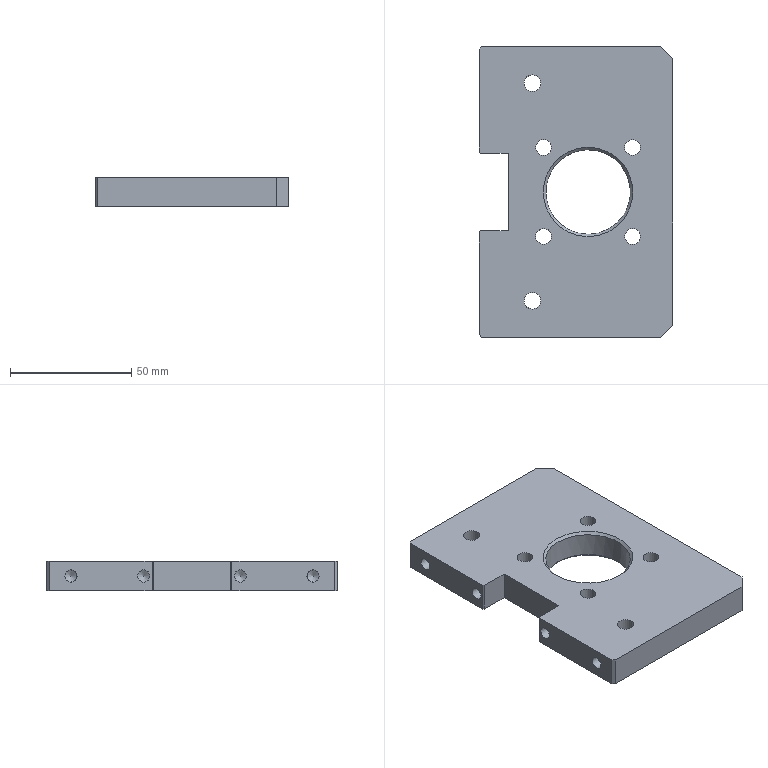NC program | NX | posted with a generic post | part box 80 x 120 x 12 mm
Whole program:
N10 G17 G21 G94 G90
(DRILLING_COPY , TOOL : D8A45)
N12 T06 M6
N14 G54
N16 G17 G0 G90 X-45. Y-18. B0. C0. S3500 M3
N18 G43 Z30. H6
N20 G94 G81 G98 Z-2.6 F250. R3.
N22 X0. Y5.
N24 X18.385 Y23.385
N26 Y-13.385
N28 X-18.385
N30 Y23.385
N32 X45. Y-18.
N34 G80
N36 G0 X45. Y-18. Z30.
N38 M5
(DRILLING_1_COPY , TOOL : 6.8ZT)
N40 T15 M6
N42 G54
N44 G17 G0 G90 X-45. Y-18. B0. C0. S2000 M3
N46 G43 Z30. H15
N48 G94 G83 G98 Z-15.543 F200. Q3. R3.
N50 X45.
N52 G80
N54 G0 X45. Y-18. Z30.
N56 M5
(DRILLING_1_COPY_COPY , TOOL : 6.5ZT)
N58 T22 M6
N60 G54
N62 G17 G0 G90 X18.385 Y23.385 B0. C0. S2000 M3
N64 G43 Z30. H22
N66 G94 G83 G98 Z-15.453 F200. Q3. R3.
N68 Y-13.385
N70 X-18.385
N72 Y23.385
N74 G80
N76 G0 X-18.385 Y23.385 Z30.
N78 M5
(HOLE_MILLING , TOOL : D10)
N80 T04 M6
N82 G54
N84 G17 G0 G90 X0. Y5. B0. C0. S7000 M3
N86 G43 Z30. H4
N88 Z0.5
N90 G94 G3 X3.1 Y8.1 R3.1 F2000.
N92 X0. Y11.2 R3.1
N94 X0. Y11.2 Z-0.5 I0. J-6.2
N96 X0. Y11.2 Z-1.5 I0. J-6.2
N98 X0. Y11.2 Z-2.5 I0. J-6.2
N100 X0. Y11.2 Z-3.5 I0. J-6.2
N102 X0. Y11.2 Z-4.5 I0. J-6.2
N104 X0. Y11.2 Z-5.5 I0. J-6.2
N106 X0. Y11.2 Z-6.5 I0. J-6.2
N108 X0. Y11.2 Z-7.5 I0. J-6.2
N110 X0. Y11.2 Z-8.5 I0. J-6.2
N112 X0. Y11.2 Z-9.5 I0. J-6.2
N114 X0. Y11.2 Z-10.5 I0. J-6.2
N116 X0. Y11.2 Z-11.5 I0. J-6.2
N118 X0. Y-1.2 Z-12. I0. J-6.2
N120 X6.2 Y5. R6.2
N122 X0. Y-1.2 R-6.2
N124 X3.1 Y1.9 R3.1
N126 X0. Y5. R3.1
N128 G0 Z0.5
N130 G3 X6.2 Y11.2 R6.2
N132 X0. Y17.4 R6.2
N134 X0. Y17.4 Z-0.5 I0. J-12.4
N136 X0. Y17.4 Z-1.5 I0. J-12.4
N138 X0. Y17.4 Z-2.5 I0. J-12.4
N140 X0. Y17.4 Z-3.5 I0. J-12.4
N142 X0. Y17.4 Z-4.5 I0. J-12.4
N144 X0. Y17.4 Z-5.5 I0. J-12.4
N146 X0. Y17.4 Z-6.5 I0. J-12.4
N148 X0. Y17.4 Z-7.5 I0. J-12.4
N150 X0. Y17.4 Z-8.5 I0. J-12.4
N152 X0. Y17.4 Z-9.5 I0. J-12.4
N154 X0. Y17.4 Z-10.5 I0. J-12.4
N156 X0. Y17.4 Z-11.5 I0. J-12.4
N158 X0. Y-7.4 Z-12. I0. J-12.4
N160 X12.4 Y5. R12.4
N162 X0. Y-7.4 R-12.4
N164 X6.2 Y-1.2 R6.2
N166 X0. Y5. R6.2
N168 G0 Z30.
(HOLE_MILLING_COPY , TOOL : D10)
N170 Z0.5
N172 G1 X2.609 Y14.031 F1200.
N174 G3 X0. Y17.5 R2.716
N176 X0. Y17.5 Z-3. I0. J-12.5
N178 X0. Y17.5 Z-6.5 I0. J-12.5
N180 X0. Y17.5 Z-10. I0. J-12.5
N182 X5.424 Y-6.262 Z-12. R-12.5
N184 X11.262 Y10.424 R12.5
N186 X5.424 Y-6.262 R-12.5
N188 X6.269 Y-2.004 R2.716
N190 G1 X0. Y5.
N192 G0 Z30.
N194 M5
(PLANAR_MILL_COPY , TOOL : D8A45)
N196 T06 M6
N198 G54
N200 G17 G0 G90 X-46.5 Y-17.134 B0. C0. S7000 M3
N202 G43 Z30. H6
N204 Z0.
N206 G94 G1 Z-1.5 F1250.
N208 G3 X-47. Y-18. R1.
N210 X-45. Y-20. R2.
N212 X-47. Y-18. R-2.
N214 X-46.5 Y-18.866 R1.
N216 G1 Z0.
N218 G0 Z30.
N220 X-19.251 Y-14.735
N222 Z0.
N224 G1 Z-1.5
N226 G3 X-18.385 Y-15.235 R1.
N228 X-16.535 Y-13.385 R1.85
N230 X-18.385 Y-15.235 R-1.85
N232 X-17.519 Y-14.735 R1.
N234 G1 Z0.
N236 G0 Z30.
N238 X-0.866 Y41.9
N240 Z0.
N242 G1 Z-1.5
N244 G3 X0. Y41.4 R1.
N246 G1 X55.
N248 G2 X55.99 Y40.99 R1.4
N250 G1 X60.99 Y35.99
N252 G2 X61.4 Y35. R1.4
N254 G1 Y-39.
N256 G2 X60.99 Y-39.99 R1.4
N258 G1 X59.99 Y-40.99
N260 G2 X59. Y-41.4 R1.4
N262 G1 X16.5
N264 G2 X15.51 Y-40.99 R1.4
N266 G1 X15.01 Y-40.49
N268 G2 X14.6 Y-39.5 R1.4
N270 G1 Y-29.4
N272 X-14.6
N274 Y-39.5
N276 G2 X-15.01 Y-40.49 R1.4
N278 G1 X-15.51 Y-40.99
N280 G2 X-16.5 Y-41.4 R1.4
N282 G1 X-59.
N284 G2 X-59.99 Y-40.99 R1.4
N286 G1 X-60.99 Y-39.99
N288 G2 X-61.4 Y-39. R1.4
N290 G1 Y35.
N292 G2 X-60.99 Y35.99 R1.4
N294 G1 X-55.99 Y40.99
N296 G2 X-55. Y41.4 R1.4
N298 G1 X0.
N300 G3 X0.866 Y41.9 R1.
N302 G1 Z0.
N304 G0 Z30.
N306 Y21.6
N308 Z0.
N310 G1 Z-1.5
N312 G3 X0. Y22.1 R1.
N314 X-17.1 Y5. R17.1
N316 X0. Y22.1 R-17.1
N318 X-0.866 Y21.6 R1.
N320 G1 Z0.
N322 G0 Z30.
N324 X-17.519 Y24.735
N326 Z0.
N328 G1 Z-1.5
N330 G3 X-18.385 Y25.235 R1.
N332 X-20.235 Y23.385 R1.85
N334 X-18.385 Y25.235 R-1.85
N336 X-19.251 Y24.735 R1.
N338 G1 Z0.
N340 G0 Z30.
N342 X19.251
N344 Z0.
N346 G1 Z-1.5
N348 G3 X18.385 Y25.235 R1.
N350 X16.535 Y23.385 R1.85
N352 X18.385 Y25.235 R-1.85
N354 X17.519 Y24.735 R1.
N356 G1 Z0.
N358 G0 Z30.
N360 Y-14.735
N362 Z0.
N364 G1 Z-1.5
N366 G3 X18.385 Y-15.235 R1.
N368 X20.235 Y-13.385 R1.85
N370 X18.385 Y-15.235 R-1.85
N372 X19.251 Y-14.735 R1.
N374 G1 Z0.
N376 G0 Z30.
N378 X46.5 Y-18.866
N380 Z0.
N382 G1 Z-1.5
N384 G3 X47. Y-18. R1.
N386 X45. Y-16. R2.
N388 X47. Y-18. R-2.
N390 X46.5 Y-17.134 R1.
N392 G1 Z0.
N394 G0 Z30.
N396 M5
N398 M2